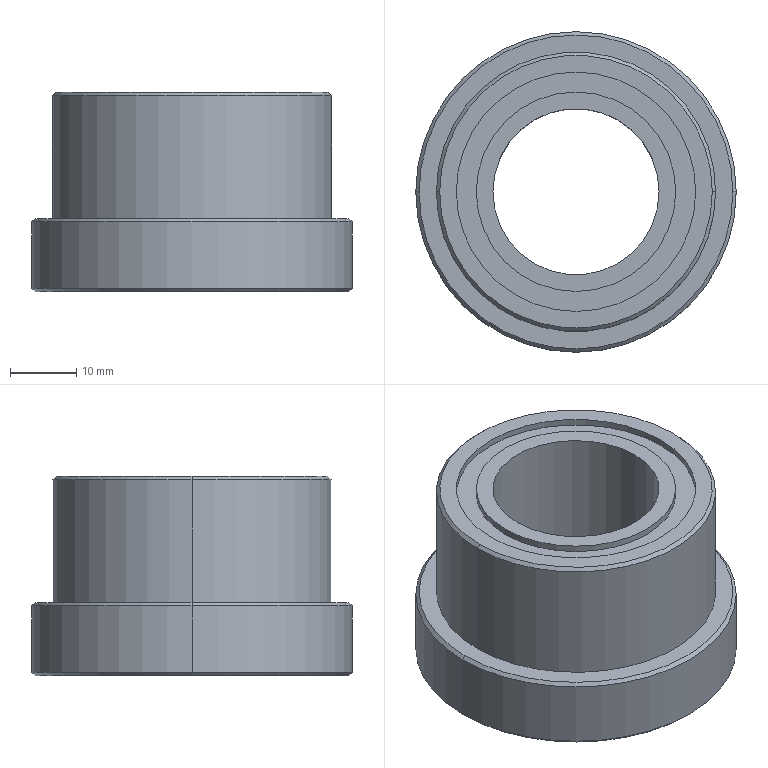Part | SolidWorks | features ICE 3, Chamfer 1, Extrusion 1 | 1 solid | 24 faces | box 48.2 x 48.2 x 30 mm | volume 28928 mm3 | cylinder 12 | cone 6 | plane 6 | commonest cylinder face diameters 30 x4 25 x2 36 x2 42 x2 48.2 x2
STEP:
#1=CARTESIAN_POINT('',(15.,0.,29.));
#2=VERTEX_POINT('',#1);
#3=CARTESIAN_POINT('',(-15.,0.,29.));
#4=VERTEX_POINT('',#3);
#5=CARTESIAN_POINT('',(0.,0.,29.));
#6=DIRECTION('',(0.,0.,1.));
#7=DIRECTION('',(1.,0.,0.));
#8=AXIS2_PLACEMENT_3D('',#5,#6,#7);
#9=CIRCLE('',#8,15.);
#10=EDGE_CURVE('',#2,#4,#9,.T.);
#11=ORIENTED_EDGE('',*,*,#10,.T.);
#12=CARTESIAN_POINT('',(-15.,0.,30.));
#13=VERTEX_POINT('',#12);
#14=CARTESIAN_POINT('',(-15.,0.,29.));
#15=DIRECTION('',(0.,0.,1.));
#16=VECTOR('',#15,1000.);
#17=LINE('',#14,#16);
#18=EDGE_CURVE('',#4,#13,#17,.T.);
#19=ORIENTED_EDGE('',*,*,#18,.T.);
#20=CARTESIAN_POINT('',(15.,0.,30.));
#21=VERTEX_POINT('',#20);
#22=CARTESIAN_POINT('',(0.,0.,30.));
#23=DIRECTION('',(0.,0.,1.));
#24=DIRECTION('',(1.,0.,0.));
#25=AXIS2_PLACEMENT_3D('',#22,#23,#24);
#26=CIRCLE('',#25,15.);
#27=EDGE_CURVE('',#21,#13,#26,.T.);
#28=ORIENTED_EDGE('',*,*,#27,.F.);
#29=CARTESIAN_POINT('',(15.,0.,29.));
#30=DIRECTION('',(0.,0.,1.));
#31=VECTOR('',#30,1000.);
#32=LINE('',#29,#31);
#33=EDGE_CURVE('',#2,#21,#32,.T.);
#34=ORIENTED_EDGE('',*,*,#33,.F.);
#35=EDGE_LOOP('',(#11,#19,#28,#34));
#36=FACE_OUTER_BOUND('',#35,.T.);
#37=CARTESIAN_POINT('',(0.,0.,29.));
#38=DIRECTION('',(0.,0.,1.));
#39=DIRECTION('',(1.,0.,0.));
#40=AXIS2_PLACEMENT_3D('',#37,#38,#39);
#41=CYLINDRICAL_SURFACE('',#40,15.);
#42=ADVANCED_FACE('',(#36),#41,.T.);
#43=CARTESIAN_POINT('',(-18.,0.,29.));
#44=VERTEX_POINT('',#43);
#45=CARTESIAN_POINT('',(18.,0.,29.));
#46=VERTEX_POINT('',#45);
#47=CARTESIAN_POINT('',(0.,0.,29.));
#48=DIRECTION('',(0.,0.,1.));
#49=DIRECTION('',(1.,0.,0.));
#50=AXIS2_PLACEMENT_3D('',#47,#48,#49);
#51=CIRCLE('',#50,18.);
#52=EDGE_CURVE('',#44,#46,#51,.T.);
#53=ORIENTED_EDGE('',*,*,#52,.F.);
#54=CARTESIAN_POINT('',(-18.,0.,30.));
#55=VERTEX_POINT('',#54);
#56=CARTESIAN_POINT('',(-18.,0.,29.));
#57=DIRECTION('',(0.,0.,1.));
#58=VECTOR('',#57,1000.);
#59=LINE('',#56,#58);
#60=EDGE_CURVE('',#44,#55,#59,.T.);
#61=ORIENTED_EDGE('',*,*,#60,.T.);
#62=CARTESIAN_POINT('',(18.,0.,30.));
#63=VERTEX_POINT('',#62);
#64=CARTESIAN_POINT('',(0.,0.,30.));
#65=DIRECTION('',(0.,0.,1.));
#66=DIRECTION('',(1.,0.,0.));
#67=AXIS2_PLACEMENT_3D('',#64,#65,#66);
#68=CIRCLE('',#67,18.);
#69=EDGE_CURVE('',#55,#63,#68,.T.);
#70=ORIENTED_EDGE('',*,*,#69,.T.);
#71=CARTESIAN_POINT('',(18.,0.,29.));
#72=DIRECTION('',(0.,0.,1.));
#73=VECTOR('',#72,1000.);
#74=LINE('',#71,#73);
#75=EDGE_CURVE('',#46,#63,#74,.T.);
#76=ORIENTED_EDGE('',*,*,#75,.F.);
#77=EDGE_LOOP('',(#53,#61,#70,#76));
#78=FACE_OUTER_BOUND('',#77,.T.);
#79=CARTESIAN_POINT('',(0.,0.,29.));
#80=DIRECTION('',(0.,0.,1.));
#81=DIRECTION('',(1.,0.,0.));
#82=AXIS2_PLACEMENT_3D('',#79,#80,#81);
#83=CYLINDRICAL_SURFACE('',#82,18.);
#84=ADVANCED_FACE('',(#78),#83,.F.);
#85=CARTESIAN_POINT('',(-23.6,0.,0.));
#86=VERTEX_POINT('',#85);
#87=CARTESIAN_POINT('',(23.6,0.,0.));
#88=VERTEX_POINT('',#87);
#89=CARTESIAN_POINT('',(0.,0.,0.));
#90=DIRECTION('',(0.,0.,-1.));
#91=DIRECTION('',(1.,0.,0.));
#92=AXIS2_PLACEMENT_3D('',#89,#90,#91);
#93=CIRCLE('',#92,23.6);
#94=EDGE_CURVE('',#86,#88,#93,.T.);
#95=ORIENTED_EDGE('',*,*,#94,.F.);
#96=CARTESIAN_POINT('',(-24.1,0.,0.5));
#97=VERTEX_POINT('',#96);
#98=CARTESIAN_POINT('',(-24.1,0.,0.5));
#99=DIRECTION('',(-0.7071,0.,0.7071));
#100=VECTOR('',#99,1000.);
#101=LINE('',#98,#100);
#102=EDGE_CURVE('',#86,#97,#101,.T.);
#103=ORIENTED_EDGE('',*,*,#102,.T.);
#104=CARTESIAN_POINT('',(24.1,0.,0.5));
#105=VERTEX_POINT('',#104);
#106=CARTESIAN_POINT('',(0.,0.,0.5));
#107=DIRECTION('',(0.,0.,1.));
#108=DIRECTION('',(1.,0.,0.));
#109=AXIS2_PLACEMENT_3D('',#106,#107,#108);
#110=CIRCLE('',#109,24.1);
#111=EDGE_CURVE('',#105,#97,#110,.T.);
#112=ORIENTED_EDGE('',*,*,#111,.F.);
#113=CARTESIAN_POINT('',(24.1,0.,0.5));
#114=DIRECTION('',(0.7071,0.,0.7071));
#115=VECTOR('',#114,1000.);
#116=LINE('',#113,#115);
#117=EDGE_CURVE('',#88,#105,#116,.T.);
#118=ORIENTED_EDGE('',*,*,#117,.F.);
#119=EDGE_LOOP('',(#95,#103,#112,#118));
#120=FACE_OUTER_BOUND('',#119,.T.);
#121=CARTESIAN_POINT('',(0.,0.,0.5));
#122=DIRECTION('',(0.,0.,1.));
#123=DIRECTION('',(1.,0.,0.));
#124=AXIS2_PLACEMENT_3D('',#121,#122,#123);
#125=CONICAL_SURFACE('',#124,24.1,0.7854);
#126=ADVANCED_FACE('',(#120),#125,.T.);
#127=CARTESIAN_POINT('',(23.6,0.,11.));
#128=VERTEX_POINT('',#127);
#129=CARTESIAN_POINT('',(-23.6,0.,11.));
#130=VERTEX_POINT('',#129);
#131=CARTESIAN_POINT('',(0.,0.,11.));
#132=DIRECTION('',(0.,0.,1.));
#133=DIRECTION('',(1.,0.,0.));
#134=AXIS2_PLACEMENT_3D('',#131,#132,#133);
#135=CIRCLE('',#134,23.6);
#136=EDGE_CURVE('',#128,#130,#135,.T.);
#137=ORIENTED_EDGE('',*,*,#136,.F.);
#138=CARTESIAN_POINT('',(24.1,0.,10.5));
#139=VERTEX_POINT('',#138);
#140=CARTESIAN_POINT('',(23.6,0.,11.));
#141=DIRECTION('',(0.7071,0.,-0.7071));
#142=VECTOR('',#141,1000.);
#143=LINE('',#140,#142);
#144=EDGE_CURVE('',#128,#139,#143,.T.);
#145=ORIENTED_EDGE('',*,*,#144,.T.);
#146=CARTESIAN_POINT('',(-24.1,0.,10.5));
#147=VERTEX_POINT('',#146);
#148=CARTESIAN_POINT('',(0.,0.,10.5));
#149=DIRECTION('',(0.,0.,-1.));
#150=DIRECTION('',(1.,0.,0.));
#151=AXIS2_PLACEMENT_3D('',#148,#149,#150);
#152=CIRCLE('',#151,24.1);
#153=EDGE_CURVE('',#147,#139,#152,.T.);
#154=ORIENTED_EDGE('',*,*,#153,.F.);
#155=CARTESIAN_POINT('',(-23.6,0.,11.));
#156=DIRECTION('',(-0.7071,0.,-0.7071));
#157=VECTOR('',#156,1000.);
#158=LINE('',#155,#157);
#159=EDGE_CURVE('',#130,#147,#158,.T.);
#160=ORIENTED_EDGE('',*,*,#159,.F.);
#161=EDGE_LOOP('',(#137,#145,#154,#160));
#162=FACE_OUTER_BOUND('',#161,.T.);
#163=CARTESIAN_POINT('',(0.,0.,11.));
#164=DIRECTION('',(0.,0.,-1.));
#165=DIRECTION('',(-1.,0.,0.));
#166=AXIS2_PLACEMENT_3D('',#163,#164,#165);
#167=CONICAL_SURFACE('',#166,23.6,0.7854);
#168=ADVANCED_FACE('',(#162),#167,.T.);
#169=CARTESIAN_POINT('',(20.5,0.,30.));
#170=VERTEX_POINT('',#169);
#171=CARTESIAN_POINT('',(-20.5,0.,30.));
#172=VERTEX_POINT('',#171);
#173=CARTESIAN_POINT('',(0.,0.,30.));
#174=DIRECTION('',(0.,0.,1.));
#175=DIRECTION('',(1.,0.,0.));
#176=AXIS2_PLACEMENT_3D('',#173,#174,#175);
#177=CIRCLE('',#176,20.5);
#178=EDGE_CURVE('',#170,#172,#177,.T.);
#179=ORIENTED_EDGE('',*,*,#178,.F.);
#180=CARTESIAN_POINT('',(21.,0.,29.5));
#181=VERTEX_POINT('',#180);
#182=CARTESIAN_POINT('',(20.5,0.,30.));
#183=DIRECTION('',(0.7071,0.,-0.7071));
#184=VECTOR('',#183,1000.);
#185=LINE('',#182,#184);
#186=EDGE_CURVE('',#170,#181,#185,.T.);
#187=ORIENTED_EDGE('',*,*,#186,.T.);
#188=CARTESIAN_POINT('',(-21.,0.,29.5));
#189=VERTEX_POINT('',#188);
#190=CARTESIAN_POINT('',(0.,0.,29.5));
#191=DIRECTION('',(0.,0.,-1.));
#192=DIRECTION('',(1.,0.,0.));
#193=AXIS2_PLACEMENT_3D('',#190,#191,#192);
#194=CIRCLE('',#193,21.);
#195=EDGE_CURVE('',#189,#181,#194,.T.);
#196=ORIENTED_EDGE('',*,*,#195,.F.);
#197=CARTESIAN_POINT('',(-20.5,0.,30.));
#198=DIRECTION('',(-0.7071,0.,-0.7071));
#199=VECTOR('',#198,1000.);
#200=LINE('',#197,#199);
#201=EDGE_CURVE('',#172,#189,#200,.T.);
#202=ORIENTED_EDGE('',*,*,#201,.F.);
#203=EDGE_LOOP('',(#179,#187,#196,#202));
#204=FACE_OUTER_BOUND('',#203,.T.);
#205=CARTESIAN_POINT('',(0.,0.,30.));
#206=DIRECTION('',(0.,0.,-1.));
#207=DIRECTION('',(-1.,0.,0.));
#208=AXIS2_PLACEMENT_3D('',#205,#206,#207);
#209=CONICAL_SURFACE('',#208,20.5,0.7854);
#210=ADVANCED_FACE('',(#204),#209,.T.);
#211=CARTESIAN_POINT('',(-12.5,0.,30.));
#212=VERTEX_POINT('',#211);
#213=CARTESIAN_POINT('',(12.5,0.,30.));
#214=VERTEX_POINT('',#213);
#215=CARTESIAN_POINT('',(0.,0.,30.));
#216=DIRECTION('',(0.,0.,1.));
#217=DIRECTION('',(1.,0.,0.));
#218=AXIS2_PLACEMENT_3D('',#215,#216,#217);
#219=CIRCLE('',#218,12.5);
#220=EDGE_CURVE('',#212,#214,#219,.T.);
#221=ORIENTED_EDGE('',*,*,#220,.T.);
#222=CARTESIAN_POINT('',(12.5,0.,11.));
#223=VERTEX_POINT('',#222);
#224=CARTESIAN_POINT('',(12.5,0.,30.));
#225=DIRECTION('',(0.,0.,-1.));
#226=VECTOR('',#225,1000.);
#227=LINE('',#224,#226);
#228=EDGE_CURVE('',#214,#223,#227,.T.);
#229=ORIENTED_EDGE('',*,*,#228,.T.);
#230=CARTESIAN_POINT('',(-12.5,0.,11.));
#231=VERTEX_POINT('',#230);
#232=CARTESIAN_POINT('',(0.,0.,11.));
#233=DIRECTION('',(0.,0.,1.));
#234=DIRECTION('',(1.,0.,0.));
#235=AXIS2_PLACEMENT_3D('',#232,#233,#234);
#236=CIRCLE('',#235,12.5);
#237=EDGE_CURVE('',#231,#223,#236,.T.);
#238=ORIENTED_EDGE('',*,*,#237,.F.);
#239=CARTESIAN_POINT('',(-12.5,0.,30.));
#240=DIRECTION('',(0.,0.,-1.));
#241=VECTOR('',#240,1000.);
#242=LINE('',#239,#241);
#243=EDGE_CURVE('',#212,#231,#242,.T.);
#244=ORIENTED_EDGE('',*,*,#243,.F.);
#245=EDGE_LOOP('',(#221,#229,#238,#244));
#246=FACE_OUTER_BOUND('',#245,.T.);
#247=CARTESIAN_POINT('',(0.,0.,30.));
#248=DIRECTION('',(0.,0.,-1.));
#249=DIRECTION('',(-1.,0.,0.));
#250=AXIS2_PLACEMENT_3D('',#247,#248,#249);
#251=CYLINDRICAL_SURFACE('',#250,12.5);
#252=ADVANCED_FACE('',(#246),#251,.F.);
#253=ORIENTED_EDGE('',*,*,#195,.T.);
#254=CARTESIAN_POINT('',(21.,0.,11.));
#255=VERTEX_POINT('',#254);
#256=CARTESIAN_POINT('',(21.,0.,30.));
#257=DIRECTION('',(0.,0.,-1.));
#258=VECTOR('',#257,1000.);
#259=LINE('',#256,#258);
#260=EDGE_CURVE('',#181,#255,#259,.T.);
#261=ORIENTED_EDGE('',*,*,#260,.T.);
#262=CARTESIAN_POINT('',(-21.,0.,11.));
#263=VERTEX_POINT('',#262);
#264=CARTESIAN_POINT('',(0.,0.,11.));
#265=DIRECTION('',(0.,0.,1.));
#266=DIRECTION('',(1.,0.,0.));
#267=AXIS2_PLACEMENT_3D('',#264,#265,#266);
#268=CIRCLE('',#267,21.);
#269=EDGE_CURVE('',#255,#263,#268,.T.);
#270=ORIENTED_EDGE('',*,*,#269,.T.);
#271=CARTESIAN_POINT('',(-21.,0.,30.));
#272=DIRECTION('',(0.,0.,-1.));
#273=VECTOR('',#272,1000.);
#274=LINE('',#271,#273);
#275=EDGE_CURVE('',#189,#263,#274,.T.);
#276=ORIENTED_EDGE('',*,*,#275,.F.);
#277=EDGE_LOOP('',(#253,#261,#270,#276));
#278=FACE_OUTER_BOUND('',#277,.T.);
#279=CARTESIAN_POINT('',(0.,0.,30.));
#280=DIRECTION('',(0.,0.,-1.));
#281=DIRECTION('',(-1.,0.,0.));
#282=AXIS2_PLACEMENT_3D('',#279,#280,#281);
#283=CYLINDRICAL_SURFACE('',#282,21.);
#284=ADVANCED_FACE('',(#278),#283,.T.);
#285=CARTESIAN_POINT('',(-15.,0.,0.));
#286=VERTEX_POINT('',#285);
#287=CARTESIAN_POINT('',(15.,0.,0.));
#288=VERTEX_POINT('',#287);
#289=CARTESIAN_POINT('',(0.,0.,0.));
#290=DIRECTION('',(0.,0.,1.));
#291=DIRECTION('',(1.,0.,0.));
#292=AXIS2_PLACEMENT_3D('',#289,#290,#291);
#293=CIRCLE('',#292,15.);
#294=EDGE_CURVE('',#286,#288,#293,.T.);
#295=ORIENTED_EDGE('',*,*,#294,.F.);
#296=CARTESIAN_POINT('',(-15.,0.,11.));
#297=VERTEX_POINT('',#296);
#298=CARTESIAN_POINT('',(-15.,0.,0.));
#299=DIRECTION('',(0.,0.,1.));
#300=VECTOR('',#299,1000.);
#301=LINE('',#298,#300);
#302=EDGE_CURVE('',#286,#297,#301,.T.);
#303=ORIENTED_EDGE('',*,*,#302,.T.);
#304=CARTESIAN_POINT('',(15.,0.,11.));
#305=VERTEX_POINT('',#304);
#306=CARTESIAN_POINT('',(0.,0.,11.));
#307=DIRECTION('',(0.,0.,-1.));
#308=DIRECTION('',(1.,0.,0.));
#309=AXIS2_PLACEMENT_3D('',#306,#307,#308);
#310=CIRCLE('',#309,15.);
#311=EDGE_CURVE('',#305,#297,#310,.T.);
#312=ORIENTED_EDGE('',*,*,#311,.F.);
#313=CARTESIAN_POINT('',(15.,0.,0.));
#314=DIRECTION('',(0.,0.,1.));
#315=VECTOR('',#314,1000.);
#316=LINE('',#313,#315);
#317=EDGE_CURVE('',#288,#305,#316,.T.);
#318=ORIENTED_EDGE('',*,*,#317,.F.);
#319=EDGE_LOOP('',(#295,#303,#312,#318));
#320=FACE_OUTER_BOUND('',#319,.T.);
#321=CARTESIAN_POINT('',(0.,0.,0.));
#322=DIRECTION('',(0.,0.,1.));
#323=DIRECTION('',(1.,0.,0.));
#324=AXIS2_PLACEMENT_3D('',#321,#322,#323);
#325=CYLINDRICAL_SURFACE('',#324,15.);
#326=ADVANCED_FACE('',(#320),#325,.F.);
#327=ORIENTED_EDGE('',*,*,#153,.T.);
#328=CARTESIAN_POINT('',(24.1,0.,11.));
#329=DIRECTION('',(0.,0.,-1.));
#330=VECTOR('',#329,1000.);
#331=LINE('',#328,#330);
#332=EDGE_CURVE('',#139,#105,#331,.T.);
#333=ORIENTED_EDGE('',*,*,#332,.T.);
#334=ORIENTED_EDGE('',*,*,#111,.T.);
#335=CARTESIAN_POINT('',(-24.1,0.,11.));
#336=DIRECTION('',(0.,0.,-1.));
#337=VECTOR('',#336,1000.);
#338=LINE('',#335,#337);
#339=EDGE_CURVE('',#147,#97,#338,.T.);
#340=ORIENTED_EDGE('',*,*,#339,.F.);
#341=EDGE_LOOP('',(#327,#333,#334,#340));
#342=FACE_OUTER_BOUND('',#341,.T.);
#343=CARTESIAN_POINT('',(0.,0.,11.));
#344=DIRECTION('',(0.,0.,-1.));
#345=DIRECTION('',(-1.,0.,0.));
#346=AXIS2_PLACEMENT_3D('',#343,#344,#345);
#347=CYLINDRICAL_SURFACE('',#346,24.1);
#348=ADVANCED_FACE('',(#342),#347,.T.);
#349=ORIENTED_EDGE('',*,*,#220,.F.);
#350=CARTESIAN_POINT('',(0.,0.,30.));
#351=DIRECTION('',(0.,0.,1.));
#352=DIRECTION('',(1.,0.,0.));
#353=AXIS2_PLACEMENT_3D('',#350,#351,#352);
#354=CIRCLE('',#353,12.5);
#355=EDGE_CURVE('',#214,#212,#354,.T.);
#356=ORIENTED_EDGE('',*,*,#355,.F.);
#357=EDGE_LOOP('',(#349,#356));
#358=FACE_BOUND('',#357,.T.);
#359=ORIENTED_EDGE('',*,*,#27,.T.);
#360=CARTESIAN_POINT('',(0.,0.,30.));
#361=DIRECTION('',(0.,0.,1.));
#362=DIRECTION('',(1.,0.,0.));
#363=AXIS2_PLACEMENT_3D('',#360,#361,#362);
#364=CIRCLE('',#363,15.);
#365=EDGE_CURVE('',#13,#21,#364,.T.);
#366=ORIENTED_EDGE('',*,*,#365,.T.);
#367=EDGE_LOOP('',(#359,#366));
#368=FACE_OUTER_BOUND('',#367,.T.);
#369=CARTESIAN_POINT('',(0.,0.,30.));
#370=DIRECTION('',(0.,0.,1.));
#371=DIRECTION('',(1.,0.,0.));
#372=AXIS2_PLACEMENT_3D('',#369,#370,#371);
#373=PLANE('',#372);
#374=ADVANCED_FACE('',(#358,#368),#373,.T.);
#375=CARTESIAN_POINT('',(0.,0.,11.));
#376=DIRECTION('',(0.,0.,1.));
#377=DIRECTION('',(1.,0.,0.));
#378=AXIS2_PLACEMENT_3D('',#375,#376,#377);
#379=CIRCLE('',#378,23.6);
#380=EDGE_CURVE('',#130,#128,#379,.T.);
#381=ORIENTED_EDGE('',*,*,#380,.T.);
#382=ORIENTED_EDGE('',*,*,#136,.T.);
#383=EDGE_LOOP('',(#381,#382));
#384=FACE_OUTER_BOUND('',#383,.T.);
#385=CARTESIAN_POINT('',(0.,0.,11.));
#386=DIRECTION('',(0.,0.,1.));
#387=DIRECTION('',(1.,0.,0.));
#388=AXIS2_PLACEMENT_3D('',#385,#386,#387);
#389=CIRCLE('',#388,21.);
#390=EDGE_CURVE('',#263,#255,#389,.T.);
#391=ORIENTED_EDGE('',*,*,#390,.F.);
#392=ORIENTED_EDGE('',*,*,#269,.F.);
#393=EDGE_LOOP('',(#391,#392));
#394=FACE_BOUND('',#393,.T.);
#395=CARTESIAN_POINT('',(0.,0.,11.));
#396=DIRECTION('',(0.,0.,1.));
#397=DIRECTION('',(1.,0.,0.));
#398=AXIS2_PLACEMENT_3D('',#395,#396,#397);
#399=PLANE('',#398);
#400=ADVANCED_FACE('',(#384,#394),#399,.T.);
#401=ORIENTED_EDGE('',*,*,#332,.F.);
#402=CARTESIAN_POINT('',(0.,0.,10.5));
#403=DIRECTION('',(0.,0.,-1.));
#404=DIRECTION('',(1.,0.,0.));
#405=AXIS2_PLACEMENT_3D('',#402,#403,#404);
#406=CIRCLE('',#405,24.1);
#407=EDGE_CURVE('',#139,#147,#406,.T.);
#408=ORIENTED_EDGE('',*,*,#407,.T.);
#409=ORIENTED_EDGE('',*,*,#339,.T.);
#410=CARTESIAN_POINT('',(0.,0.,0.5));
#411=DIRECTION('',(0.,0.,1.));
#412=DIRECTION('',(1.,0.,0.));
#413=AXIS2_PLACEMENT_3D('',#410,#411,#412);
#414=CIRCLE('',#413,24.1);
#415=EDGE_CURVE('',#97,#105,#414,.T.);
#416=ORIENTED_EDGE('',*,*,#415,.T.);
#417=EDGE_LOOP('',(#401,#408,#409,#416));
#418=FACE_OUTER_BOUND('',#417,.T.);
#419=CARTESIAN_POINT('',(0.,0.,11.));
#420=DIRECTION('',(0.,0.,-1.));
#421=DIRECTION('',(-1.,0.,0.));
#422=AXIS2_PLACEMENT_3D('',#419,#420,#421);
#423=CYLINDRICAL_SURFACE('',#422,24.1);
#424=ADVANCED_FACE('',(#418),#423,.T.);
#425=CARTESIAN_POINT('',(0.,0.,0.));
#426=DIRECTION('',(0.,0.,-1.));
#427=DIRECTION('',(1.,0.,0.));
#428=AXIS2_PLACEMENT_3D('',#425,#426,#427);
#429=CIRCLE('',#428,23.6);
#430=EDGE_CURVE('',#88,#86,#429,.T.);
#431=ORIENTED_EDGE('',*,*,#430,.T.);
#432=ORIENTED_EDGE('',*,*,#94,.T.);
#433=EDGE_LOOP('',(#431,#432));
#434=FACE_OUTER_BOUND('',#433,.T.);
#435=CARTESIAN_POINT('',(0.,0.,0.));
#436=DIRECTION('',(0.,0.,1.));
#437=DIRECTION('',(1.,0.,0.));
#438=AXIS2_PLACEMENT_3D('',#435,#436,#437);
#439=CIRCLE('',#438,15.);
#440=EDGE_CURVE('',#288,#286,#439,.T.);
#441=ORIENTED_EDGE('',*,*,#440,.T.);
#442=ORIENTED_EDGE('',*,*,#294,.T.);
#443=EDGE_LOOP('',(#441,#442));
#444=FACE_BOUND('',#443,.T.);
#445=CARTESIAN_POINT('',(0.,0.,0.));
#446=DIRECTION('',(0.,0.,1.));
#447=DIRECTION('',(1.,0.,0.));
#448=AXIS2_PLACEMENT_3D('',#445,#446,#447);
#449=PLANE('',#448);
#450=ADVANCED_FACE('',(#434,#444),#449,.F.);
#451=ORIENTED_EDGE('',*,*,#302,.F.);
#452=ORIENTED_EDGE('',*,*,#440,.F.);
#453=ORIENTED_EDGE('',*,*,#317,.T.);
#454=CARTESIAN_POINT('',(0.,0.,11.));
#455=DIRECTION('',(0.,0.,-1.));
#456=DIRECTION('',(1.,0.,0.));
#457=AXIS2_PLACEMENT_3D('',#454,#455,#456);
#458=CIRCLE('',#457,15.);
#459=EDGE_CURVE('',#297,#305,#458,.T.);
#460=ORIENTED_EDGE('',*,*,#459,.F.);
#461=EDGE_LOOP('',(#451,#452,#453,#460));
#462=FACE_OUTER_BOUND('',#461,.T.);
#463=CARTESIAN_POINT('',(0.,0.,0.));
#464=DIRECTION('',(0.,0.,1.));
#465=DIRECTION('',(1.,0.,0.));
#466=AXIS2_PLACEMENT_3D('',#463,#464,#465);
#467=CYLINDRICAL_SURFACE('',#466,15.);
#468=ADVANCED_FACE('',(#462),#467,.F.);
#469=ORIENTED_EDGE('',*,*,#237,.T.);
#470=CARTESIAN_POINT('',(0.,0.,11.));
#471=DIRECTION('',(0.,0.,1.));
#472=DIRECTION('',(1.,0.,0.));
#473=AXIS2_PLACEMENT_3D('',#470,#471,#472);
#474=CIRCLE('',#473,12.5);
#475=EDGE_CURVE('',#223,#231,#474,.T.);
#476=ORIENTED_EDGE('',*,*,#475,.T.);
#477=EDGE_LOOP('',(#469,#476));
#478=FACE_BOUND('',#477,.T.);
#479=ORIENTED_EDGE('',*,*,#311,.T.);
#480=ORIENTED_EDGE('',*,*,#459,.T.);
#481=EDGE_LOOP('',(#479,#480));
#482=FACE_OUTER_BOUND('',#481,.T.);
#483=CARTESIAN_POINT('',(0.,0.,11.));
#484=DIRECTION('',(0.,0.,1.));
#485=DIRECTION('',(1.,0.,0.));
#486=AXIS2_PLACEMENT_3D('',#483,#484,#485);
#487=PLANE('',#486);
#488=ADVANCED_FACE('',(#478,#482),#487,.F.);
#489=CARTESIAN_POINT('',(0.,0.,30.));
#490=DIRECTION('',(0.,0.,1.));
#491=DIRECTION('',(1.,0.,0.));
#492=AXIS2_PLACEMENT_3D('',#489,#490,#491);
#493=CIRCLE('',#492,18.);
#494=EDGE_CURVE('',#63,#55,#493,.T.);
#495=ORIENTED_EDGE('',*,*,#494,.F.);
#496=ORIENTED_EDGE('',*,*,#69,.F.);
#497=EDGE_LOOP('',(#495,#496));
#498=FACE_BOUND('',#497,.T.);
#499=CARTESIAN_POINT('',(0.,0.,30.));
#500=DIRECTION('',(0.,0.,1.));
#501=DIRECTION('',(1.,0.,0.));
#502=AXIS2_PLACEMENT_3D('',#499,#500,#501);
#503=CIRCLE('',#502,20.5);
#504=EDGE_CURVE('',#172,#170,#503,.T.);
#505=ORIENTED_EDGE('',*,*,#504,.T.);
#506=ORIENTED_EDGE('',*,*,#178,.T.);
#507=EDGE_LOOP('',(#505,#506));
#508=FACE_OUTER_BOUND('',#507,.T.);
#509=CARTESIAN_POINT('',(0.,0.,30.));
#510=DIRECTION('',(0.,0.,1.));
#511=DIRECTION('',(1.,0.,0.));
#512=AXIS2_PLACEMENT_3D('',#509,#510,#511);
#513=PLANE('',#512);
#514=ADVANCED_FACE('',(#498,#508),#513,.T.);
#515=ORIENTED_EDGE('',*,*,#260,.F.);
#516=CARTESIAN_POINT('',(0.,0.,29.5));
#517=DIRECTION('',(0.,0.,-1.));
#518=DIRECTION('',(1.,0.,0.));
#519=AXIS2_PLACEMENT_3D('',#516,#517,#518);
#520=CIRCLE('',#519,21.);
#521=EDGE_CURVE('',#181,#189,#520,.T.);
#522=ORIENTED_EDGE('',*,*,#521,.T.);
#523=ORIENTED_EDGE('',*,*,#275,.T.);
#524=ORIENTED_EDGE('',*,*,#390,.T.);
#525=EDGE_LOOP('',(#515,#522,#523,#524));
#526=FACE_OUTER_BOUND('',#525,.T.);
#527=CARTESIAN_POINT('',(0.,0.,30.));
#528=DIRECTION('',(0.,0.,-1.));
#529=DIRECTION('',(-1.,0.,0.));
#530=AXIS2_PLACEMENT_3D('',#527,#528,#529);
#531=CYLINDRICAL_SURFACE('',#530,21.);
#532=ADVANCED_FACE('',(#526),#531,.T.);
#533=ORIENTED_EDGE('',*,*,#228,.F.);
#534=ORIENTED_EDGE('',*,*,#355,.T.);
#535=ORIENTED_EDGE('',*,*,#243,.T.);
#536=ORIENTED_EDGE('',*,*,#475,.F.);
#537=EDGE_LOOP('',(#533,#534,#535,#536));
#538=FACE_OUTER_BOUND('',#537,.T.);
#539=CARTESIAN_POINT('',(0.,0.,30.));
#540=DIRECTION('',(0.,0.,-1.));
#541=DIRECTION('',(-1.,0.,0.));
#542=AXIS2_PLACEMENT_3D('',#539,#540,#541);
#543=CYLINDRICAL_SURFACE('',#542,12.5);
#544=ADVANCED_FACE('',(#538),#543,.F.);
#545=ORIENTED_EDGE('',*,*,#186,.F.);
#546=ORIENTED_EDGE('',*,*,#504,.F.);
#547=ORIENTED_EDGE('',*,*,#201,.T.);
#548=ORIENTED_EDGE('',*,*,#521,.F.);
#549=EDGE_LOOP('',(#545,#546,#547,#548));
#550=FACE_OUTER_BOUND('',#549,.T.);
#551=CARTESIAN_POINT('',(0.,0.,30.));
#552=DIRECTION('',(0.,0.,-1.));
#553=DIRECTION('',(-1.,0.,0.));
#554=AXIS2_PLACEMENT_3D('',#551,#552,#553);
#555=CONICAL_SURFACE('',#554,20.5,0.7854);
#556=ADVANCED_FACE('',(#550),#555,.T.);
#557=ORIENTED_EDGE('',*,*,#144,.F.);
#558=ORIENTED_EDGE('',*,*,#380,.F.);
#559=ORIENTED_EDGE('',*,*,#159,.T.);
#560=ORIENTED_EDGE('',*,*,#407,.F.);
#561=EDGE_LOOP('',(#557,#558,#559,#560));
#562=FACE_OUTER_BOUND('',#561,.T.);
#563=CARTESIAN_POINT('',(0.,0.,11.));
#564=DIRECTION('',(0.,0.,-1.));
#565=DIRECTION('',(-1.,0.,0.));
#566=AXIS2_PLACEMENT_3D('',#563,#564,#565);
#567=CONICAL_SURFACE('',#566,23.6,0.7854);
#568=ADVANCED_FACE('',(#562),#567,.T.);
#569=ORIENTED_EDGE('',*,*,#102,.F.);
#570=ORIENTED_EDGE('',*,*,#430,.F.);
#571=ORIENTED_EDGE('',*,*,#117,.T.);
#572=ORIENTED_EDGE('',*,*,#415,.F.);
#573=EDGE_LOOP('',(#569,#570,#571,#572));
#574=FACE_OUTER_BOUND('',#573,.T.);
#575=CARTESIAN_POINT('',(0.,0.,0.5));
#576=DIRECTION('',(0.,0.,1.));
#577=DIRECTION('',(1.,0.,0.));
#578=AXIS2_PLACEMENT_3D('',#575,#576,#577);
#579=CONICAL_SURFACE('',#578,24.1,0.7854);
#580=ADVANCED_FACE('',(#574),#579,.T.);
#581=ORIENTED_EDGE('',*,*,#60,.F.);
#582=CARTESIAN_POINT('',(0.,0.,29.));
#583=DIRECTION('',(0.,0.,1.));
#584=DIRECTION('',(1.,0.,0.));
#585=AXIS2_PLACEMENT_3D('',#582,#583,#584);
#586=CIRCLE('',#585,18.);
#587=EDGE_CURVE('',#46,#44,#586,.T.);
#588=ORIENTED_EDGE('',*,*,#587,.F.);
#589=ORIENTED_EDGE('',*,*,#75,.T.);
#590=ORIENTED_EDGE('',*,*,#494,.T.);
#591=EDGE_LOOP('',(#581,#588,#589,#590));
#592=FACE_OUTER_BOUND('',#591,.T.);
#593=CARTESIAN_POINT('',(0.,0.,29.));
#594=DIRECTION('',(0.,0.,1.));
#595=DIRECTION('',(1.,0.,0.));
#596=AXIS2_PLACEMENT_3D('',#593,#594,#595);
#597=CYLINDRICAL_SURFACE('',#596,18.);
#598=ADVANCED_FACE('',(#592),#597,.F.);
#599=ORIENTED_EDGE('',*,*,#10,.F.);
#600=CARTESIAN_POINT('',(0.,0.,29.));
#601=DIRECTION('',(0.,0.,1.));
#602=DIRECTION('',(1.,0.,0.));
#603=AXIS2_PLACEMENT_3D('',#600,#601,#602);
#604=CIRCLE('',#603,15.);
#605=EDGE_CURVE('',#4,#2,#604,.T.);
#606=ORIENTED_EDGE('',*,*,#605,.F.);
#607=EDGE_LOOP('',(#599,#606));
#608=FACE_BOUND('',#607,.T.);
#609=ORIENTED_EDGE('',*,*,#587,.T.);
#610=ORIENTED_EDGE('',*,*,#52,.T.);
#611=EDGE_LOOP('',(#609,#610));
#612=FACE_OUTER_BOUND('',#611,.T.);
#613=CARTESIAN_POINT('',(0.,0.,29.));
#614=DIRECTION('',(0.,0.,1.));
#615=DIRECTION('',(1.,0.,0.));
#616=AXIS2_PLACEMENT_3D('',#613,#614,#615);
#617=PLANE('',#616);
#618=ADVANCED_FACE('',(#608,#612),#617,.T.);
#619=ORIENTED_EDGE('',*,*,#18,.F.);
#620=ORIENTED_EDGE('',*,*,#605,.T.);
#621=ORIENTED_EDGE('',*,*,#33,.T.);
#622=ORIENTED_EDGE('',*,*,#365,.F.);
#623=EDGE_LOOP('',(#619,#620,#621,#622));
#624=FACE_OUTER_BOUND('',#623,.T.);
#625=CARTESIAN_POINT('',(0.,0.,29.));
#626=DIRECTION('',(0.,0.,1.));
#627=DIRECTION('',(1.,0.,0.));
#628=AXIS2_PLACEMENT_3D('',#625,#626,#627);
#629=CYLINDRICAL_SURFACE('',#628,15.);
#630=ADVANCED_FACE('',(#624),#629,.T.);
#631=CLOSED_SHELL('',(#42,#84,#126,#168,#210,#252,#284,#326,#348,#374,#400,#424,#450,#468,#488,#514,#532,#544,#556,#568,#580,#598,#618,#630));
#632=MANIFOLD_SOLID_BREP('',#631);
#633=CARTESIAN_POINT('',(0.,0.,0.));
#634=DIRECTION('',(0.,0.,1.));
#635=DIRECTION('',(1.,0.,0.));
#636=AXIS2_PLACEMENT_3D('',#633,#634,#635);
#637=(LENGTH_UNIT()NAMED_UNIT(*)SI_UNIT(.MILLI.,.METRE.));
#638=UNCERTAINTY_MEASURE_WITH_UNIT(LENGTH_MEASURE(0.00001),#637,'','');
#639=(NAMED_UNIT(*)PLANE_ANGLE_UNIT()SI_UNIT($,.RADIAN.));
#640=(NAMED_UNIT(*)SI_UNIT($,.STERADIAN.)SOLID_ANGLE_UNIT());
#641=(GEOMETRIC_REPRESENTATION_CONTEXT(3)GLOBAL_UNCERTAINTY_ASSIGNED_CONTEXT((#638))GLOBAL_UNIT_ASSIGNED_CONTEXT((#637,#639,#640))REPRESENTATION_CONTEXT('',''));
#642=ADVANCED_BREP_SHAPE_REPRESENTATION('',(#632,#636),#641);